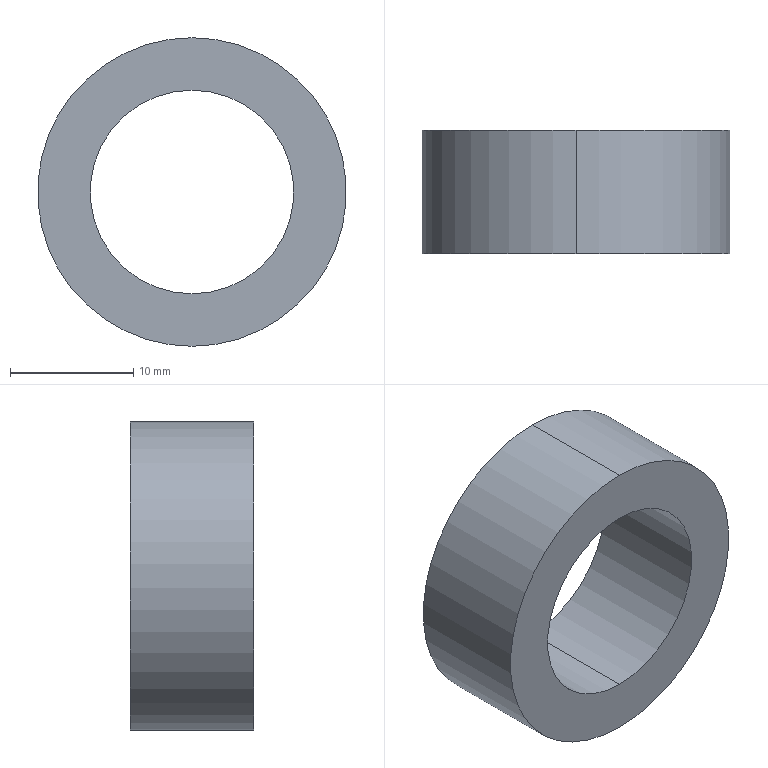Part | SolidWorks | features Extrusion 1 | 1 solid | 6 faces | box 25 x 10 x 25 mm | volume 2770 mm3 | cylinder 4 | plane 2 | commonest cylinder face diameters 16.5 x2 25 x2
STEP:
#1=CARTESIAN_POINT('',(0.,10.,-8.25));
#2=VERTEX_POINT('',#1);
#3=CARTESIAN_POINT('',(0.,10.,8.25));
#4=VERTEX_POINT('',#3);
#5=CARTESIAN_POINT('',(0.,10.,0.));
#6=DIRECTION('',(0.,1.,0.));
#7=DIRECTION('',(0.,0.,1.));
#8=AXIS2_PLACEMENT_3D('',#5,#6,#7);
#9=CIRCLE('',#8,8.25);
#10=EDGE_CURVE('',#2,#4,#9,.T.);
#11=ORIENTED_EDGE('',*,*,#10,.T.);
#12=CARTESIAN_POINT('',(0.,0.,8.25));
#13=VERTEX_POINT('',#12);
#14=CARTESIAN_POINT('',(0.,10.,8.25));
#15=DIRECTION('',(0.,-1.,0.));
#16=VECTOR('',#15,1000.);
#17=LINE('',#14,#16);
#18=EDGE_CURVE('',#4,#13,#17,.T.);
#19=ORIENTED_EDGE('',*,*,#18,.T.);
#20=CARTESIAN_POINT('',(0.,0.,-8.25));
#21=VERTEX_POINT('',#20);
#22=CARTESIAN_POINT('',(0.,0.,0.));
#23=DIRECTION('',(0.,1.,0.));
#24=DIRECTION('',(0.,0.,1.));
#25=AXIS2_PLACEMENT_3D('',#22,#23,#24);
#26=CIRCLE('',#25,8.25);
#27=EDGE_CURVE('',#21,#13,#26,.T.);
#28=ORIENTED_EDGE('',*,*,#27,.F.);
#29=CARTESIAN_POINT('',(0.,10.,-8.25));
#30=DIRECTION('',(0.,-1.,0.));
#31=VECTOR('',#30,1000.);
#32=LINE('',#29,#31);
#33=EDGE_CURVE('',#2,#21,#32,.T.);
#34=ORIENTED_EDGE('',*,*,#33,.F.);
#35=EDGE_LOOP('',(#11,#19,#28,#34));
#36=FACE_OUTER_BOUND('',#35,.T.);
#37=CARTESIAN_POINT('',(0.,10.,0.));
#38=DIRECTION('',(0.,-1.,0.));
#39=DIRECTION('',(0.,0.,-1.));
#40=AXIS2_PLACEMENT_3D('',#37,#38,#39);
#41=CYLINDRICAL_SURFACE('',#40,8.25);
#42=ADVANCED_FACE('',(#36),#41,.F.);
#43=CARTESIAN_POINT('',(0.,10.,12.5));
#44=VERTEX_POINT('',#43);
#45=CARTESIAN_POINT('',(0.,10.,-12.5));
#46=VERTEX_POINT('',#45);
#47=CARTESIAN_POINT('',(0.,10.,0.));
#48=DIRECTION('',(0.,1.,0.));
#49=DIRECTION('',(0.,0.,1.));
#50=AXIS2_PLACEMENT_3D('',#47,#48,#49);
#51=CIRCLE('',#50,12.5);
#52=EDGE_CURVE('',#44,#46,#51,.T.);
#53=ORIENTED_EDGE('',*,*,#52,.F.);
#54=CARTESIAN_POINT('',(0.,0.,12.5));
#55=VERTEX_POINT('',#54);
#56=CARTESIAN_POINT('',(0.,10.,12.5));
#57=DIRECTION('',(0.,-1.,0.));
#58=VECTOR('',#57,1000.);
#59=LINE('',#56,#58);
#60=EDGE_CURVE('',#44,#55,#59,.T.);
#61=ORIENTED_EDGE('',*,*,#60,.T.);
#62=CARTESIAN_POINT('',(0.,0.,-12.5));
#63=VERTEX_POINT('',#62);
#64=CARTESIAN_POINT('',(0.,0.,0.));
#65=DIRECTION('',(0.,1.,0.));
#66=DIRECTION('',(0.,0.,1.));
#67=AXIS2_PLACEMENT_3D('',#64,#65,#66);
#68=CIRCLE('',#67,12.5);
#69=EDGE_CURVE('',#55,#63,#68,.T.);
#70=ORIENTED_EDGE('',*,*,#69,.T.);
#71=CARTESIAN_POINT('',(0.,10.,-12.5));
#72=DIRECTION('',(0.,-1.,0.));
#73=VECTOR('',#72,1000.);
#74=LINE('',#71,#73);
#75=EDGE_CURVE('',#46,#63,#74,.T.);
#76=ORIENTED_EDGE('',*,*,#75,.F.);
#77=EDGE_LOOP('',(#53,#61,#70,#76));
#78=FACE_OUTER_BOUND('',#77,.T.);
#79=CARTESIAN_POINT('',(0.,10.,0.));
#80=DIRECTION('',(0.,-1.,0.));
#81=DIRECTION('',(0.,0.,-1.));
#82=AXIS2_PLACEMENT_3D('',#79,#80,#81);
#83=CYLINDRICAL_SURFACE('',#82,12.5);
#84=ADVANCED_FACE('',(#78),#83,.T.);
#85=CARTESIAN_POINT('',(0.,10.,0.));
#86=DIRECTION('',(0.,1.,0.));
#87=DIRECTION('',(0.,0.,1.));
#88=AXIS2_PLACEMENT_3D('',#85,#86,#87);
#89=CIRCLE('',#88,12.5);
#90=EDGE_CURVE('',#46,#44,#89,.T.);
#91=ORIENTED_EDGE('',*,*,#90,.T.);
#92=ORIENTED_EDGE('',*,*,#52,.T.);
#93=EDGE_LOOP('',(#91,#92));
#94=FACE_OUTER_BOUND('',#93,.T.);
#95=ORIENTED_EDGE('',*,*,#10,.F.);
#96=CARTESIAN_POINT('',(0.,10.,0.));
#97=DIRECTION('',(0.,1.,0.));
#98=DIRECTION('',(0.,0.,1.));
#99=AXIS2_PLACEMENT_3D('',#96,#97,#98);
#100=CIRCLE('',#99,8.25);
#101=EDGE_CURVE('',#4,#2,#100,.T.);
#102=ORIENTED_EDGE('',*,*,#101,.F.);
#103=EDGE_LOOP('',(#95,#102));
#104=FACE_BOUND('',#103,.T.);
#105=CARTESIAN_POINT('',(0.,10.,0.));
#106=DIRECTION('',(0.,1.,0.));
#107=DIRECTION('',(0.,0.,1.));
#108=AXIS2_PLACEMENT_3D('',#105,#106,#107);
#109=PLANE('',#108);
#110=ADVANCED_FACE('',(#94,#104),#109,.T.);
#111=CARTESIAN_POINT('',(0.,0.,0.));
#112=DIRECTION('',(0.,1.,0.));
#113=DIRECTION('',(0.,0.,1.));
#114=AXIS2_PLACEMENT_3D('',#111,#112,#113);
#115=CIRCLE('',#114,12.5);
#116=EDGE_CURVE('',#63,#55,#115,.T.);
#117=ORIENTED_EDGE('',*,*,#116,.F.);
#118=ORIENTED_EDGE('',*,*,#69,.F.);
#119=EDGE_LOOP('',(#117,#118));
#120=FACE_OUTER_BOUND('',#119,.T.);
#121=ORIENTED_EDGE('',*,*,#27,.T.);
#122=CARTESIAN_POINT('',(0.,0.,0.));
#123=DIRECTION('',(0.,1.,0.));
#124=DIRECTION('',(0.,0.,1.));
#125=AXIS2_PLACEMENT_3D('',#122,#123,#124);
#126=CIRCLE('',#125,8.25);
#127=EDGE_CURVE('',#13,#21,#126,.T.);
#128=ORIENTED_EDGE('',*,*,#127,.T.);
#129=EDGE_LOOP('',(#121,#128));
#130=FACE_BOUND('',#129,.T.);
#131=CARTESIAN_POINT('',(0.,0.,0.));
#132=DIRECTION('',(0.,1.,0.));
#133=DIRECTION('',(0.,0.,1.));
#134=AXIS2_PLACEMENT_3D('',#131,#132,#133);
#135=PLANE('',#134);
#136=ADVANCED_FACE('',(#120,#130),#135,.F.);
#137=ORIENTED_EDGE('',*,*,#60,.F.);
#138=ORIENTED_EDGE('',*,*,#90,.F.);
#139=ORIENTED_EDGE('',*,*,#75,.T.);
#140=ORIENTED_EDGE('',*,*,#116,.T.);
#141=EDGE_LOOP('',(#137,#138,#139,#140));
#142=FACE_OUTER_BOUND('',#141,.T.);
#143=CARTESIAN_POINT('',(0.,10.,0.));
#144=DIRECTION('',(0.,-1.,0.));
#145=DIRECTION('',(0.,0.,-1.));
#146=AXIS2_PLACEMENT_3D('',#143,#144,#145);
#147=CYLINDRICAL_SURFACE('',#146,12.5);
#148=ADVANCED_FACE('',(#142),#147,.T.);
#149=ORIENTED_EDGE('',*,*,#18,.F.);
#150=ORIENTED_EDGE('',*,*,#101,.T.);
#151=ORIENTED_EDGE('',*,*,#33,.T.);
#152=ORIENTED_EDGE('',*,*,#127,.F.);
#153=EDGE_LOOP('',(#149,#150,#151,#152));
#154=FACE_OUTER_BOUND('',#153,.T.);
#155=CARTESIAN_POINT('',(0.,10.,0.));
#156=DIRECTION('',(0.,-1.,0.));
#157=DIRECTION('',(0.,0.,-1.));
#158=AXIS2_PLACEMENT_3D('',#155,#156,#157);
#159=CYLINDRICAL_SURFACE('',#158,8.25);
#160=ADVANCED_FACE('',(#154),#159,.F.);
#161=CLOSED_SHELL('',(#42,#84,#110,#136,#148,#160));
#162=MANIFOLD_SOLID_BREP('',#161);
#163=CARTESIAN_POINT('',(0.,0.,0.));
#164=DIRECTION('',(0.,0.,1.));
#165=DIRECTION('',(1.,0.,0.));
#166=AXIS2_PLACEMENT_3D('',#163,#164,#165);
#167=(LENGTH_UNIT()NAMED_UNIT(*)SI_UNIT(.MILLI.,.METRE.));
#168=UNCERTAINTY_MEASURE_WITH_UNIT(LENGTH_MEASURE(0.00001),#167,'','');
#169=(NAMED_UNIT(*)PLANE_ANGLE_UNIT()SI_UNIT($,.RADIAN.));
#170=(NAMED_UNIT(*)SI_UNIT($,.STERADIAN.)SOLID_ANGLE_UNIT());
#171=(GEOMETRIC_REPRESENTATION_CONTEXT(3)GLOBAL_UNCERTAINTY_ASSIGNED_CONTEXT((#168))GLOBAL_UNIT_ASSIGNED_CONTEXT((#167,#169,#170))REPRESENTATION_CONTEXT('',''));
#172=ADVANCED_BREP_SHAPE_REPRESENTATION('',(#162,#166),#171);